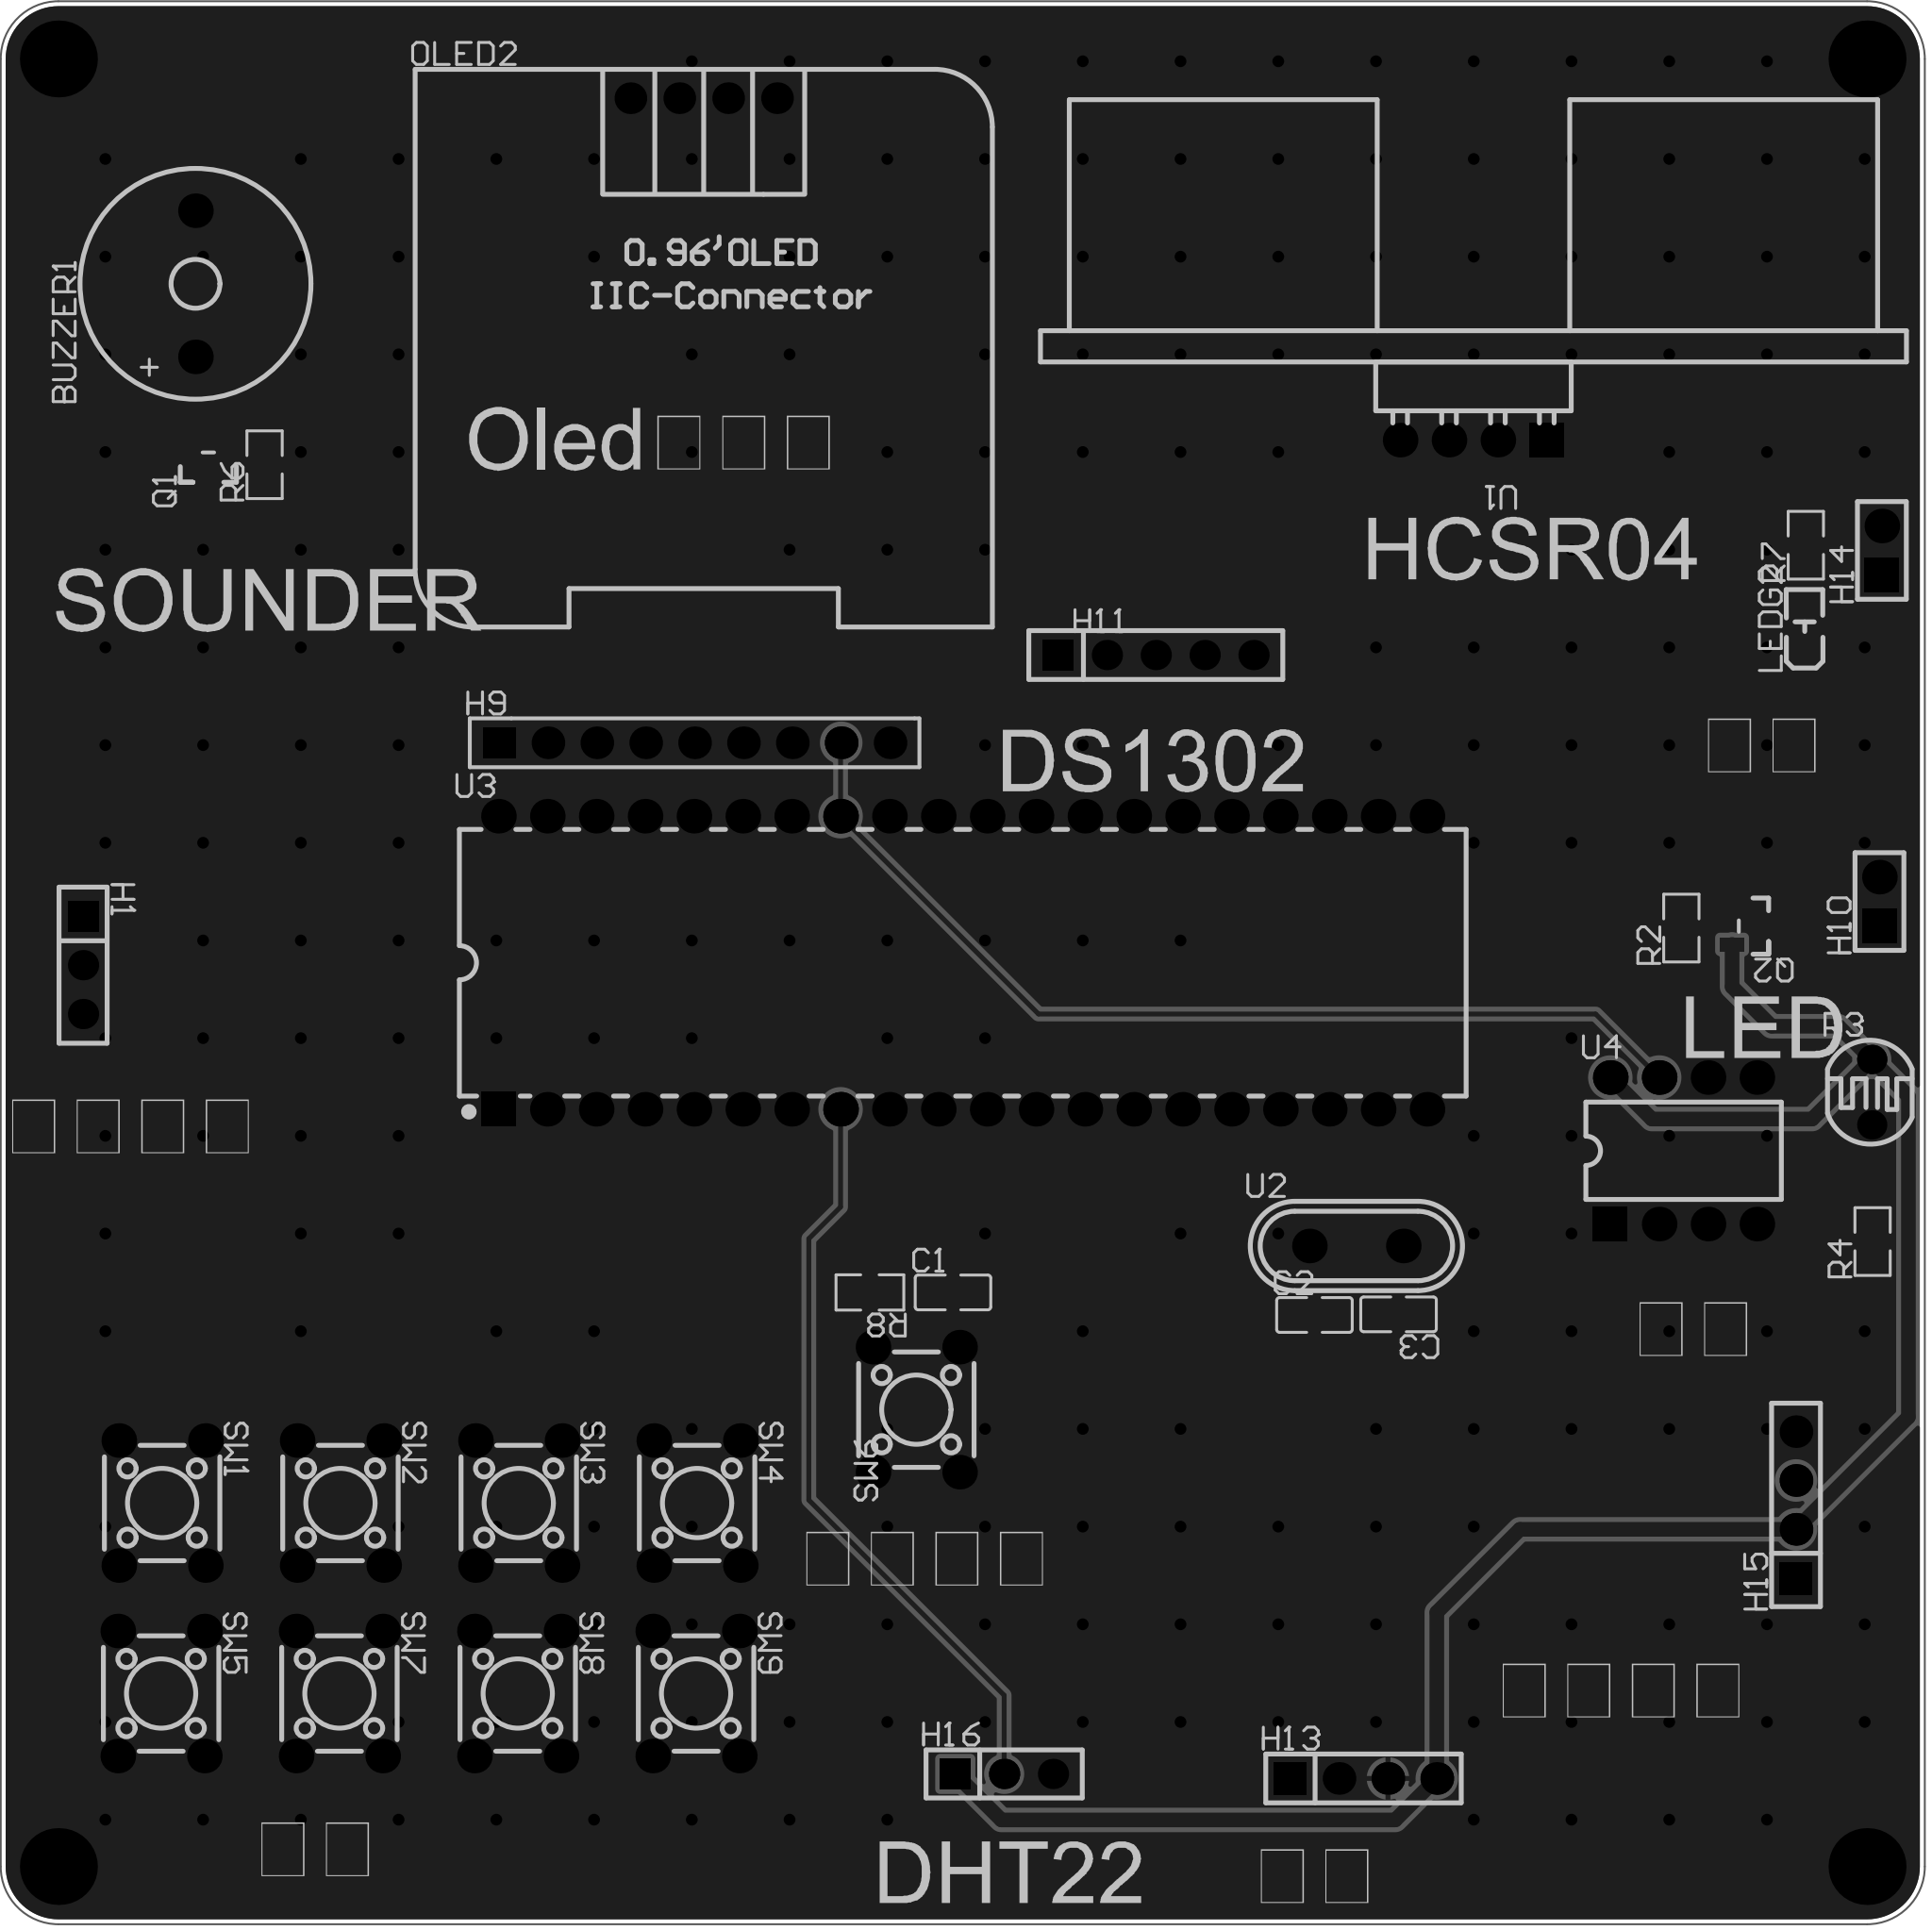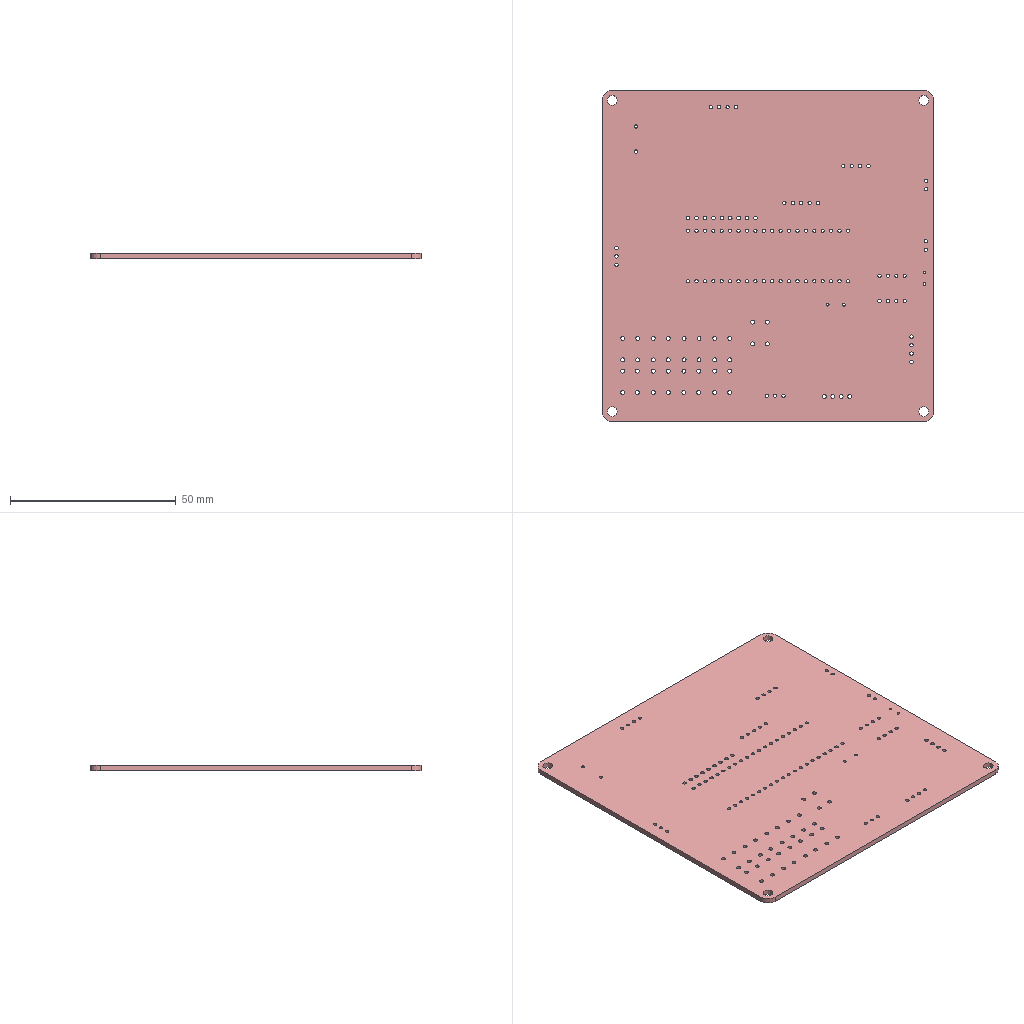Circuit board layout | Altium Designer | box 100 x 100 x 1.6 mm
Layer stack:
# Altium Designer layer stack of  (unit mm; dielectric type: 0 none, 1 core, 2 prepreg, 3 surface material)
index,name,kind,layer,copper_thickness_mm,dielectric_type,dielectric_thickness_mm,dielectric_material,dielectric_constant
0,Top Paste Mask Layer,other,,,,,,
1,Top Silkscreen Layer,other,,,,,,
2,Top Solder Mask Layer,dielectric,,,3,0.01,,3.3
3,Top Layer,copper,Top Layer,0.035,,,,
4,Dielectric1,dielectric,,,3,1.51,FR4,4.5
5,Bottom Layer,copper,Bottom Layer,0.035,,,,
6,Bottom Solder Mask Layer,dielectric,,,3,0.01,,3.3
7,Bottom Silkscreen Layer,other,,,,,,
8,Bottom Paste Mask Layer,other,,,,,,
# drill layer pairs: low layer,high layer
drill_pair,Top Layer,Bottom Layer
Part placement:
Designator,Comment,Layer,Footprint,Center-X(mm),Center-Y(mm),Rotation
SW1,,TopLayer,SW-TH_4P-L6.0-W6.0-P4.50-LS6.5,99.74,102.841,270
SW2,,TopLayer,SW-TH_4P-L6.0-W6.0-P4.50-LS6.5,109.007,102.841,270
SW3,,TopLayer,SW-TH_4P-L6.0-W6.0-P4.50-LS6.5,118.275,102.841,270
SW4,,TopLayer,SW-TH_4P-L6.0-W6.0-P4.50-LS6.5,127.543,102.841,270
OLED2,,TopLayer,0.96OLED_4P,127.889,175.895,0
BUZZER1,buzzer-12X9,TopLayer,BUZ-TH_BD12.0-P7.60-D0.6-FD,101.473,166.243,90
C1,10uf,TopLayer,C0805,140.843,113.792,0
C2,30pf,TopLayer,C0805,159.629,112.62,0
C3,30pf,TopLayer,C0805,164,112.652,180
H9,,TopLayer,HDR-TH_9P-P2.54-V-F-1,127.414,142.375,0
H13,,TopLayer,HDR-TH_4P-P2.54-V-M,162.179,88.519,0
H14,,TopLayer,HDR-TH_2P-P2.54-V-M-1,189.121,152.379,90
LEDG2,,TopLayer,LED_0805,185.106,148.363,90
Q1,2N3906S-RTK/PS,TopLayer,SOT-23-3_L2.9-W1.3-P1.90-LS2.4-TR,102.143,156.573,90
R6,2.2K,TopLayer,R0805,105.064,156.835,90
R7,220,TopLayer,R0805,185.168,152.649,90
R8,10K,TopLayer,R0805,136.525,113.792,180
U2,11.059MHz,TopLayer,HC-49US_L11.0-W4.6-P4.88,161.809,116.208,0
U3,STC89C516RD+40I-PDIP40,TopLayer,DIP-40_L52.3-W13.9-P2.54-LS15.2-BL,141.351,130.937,0
H1,,TopLayer,HDR-TH_3P-P2.54-V-F,95.631,130.81,270
H10,,TopLayer,HDR-TH_2P-P2.54-V-M-1,188.994,134.12,90
H15,,TopLayer,HDR-TH_4P-P2.54-V-F,184.658,102.743,90
H16,,TopLayer,HDR-TH_3P-P2.54-V-F,143.502,88.753,0
U1,HC-SR04,TopLayer,TH_HC-SR04V,167.894,158.115,180
Q2,,TopLayer,S8550P_SOT,182.584,132.842,180
H11,,TopLayer,HDR-TH_5P-P2.54-V-F,151.384,146.939,0
R2,1K,TopLayer,R0805,178.698,132.739,90
R3,GL5549(80-100),TopLayer,RES-TH_L5.1-W4.3-P3.40-D0.5,188.595,124.206,0
R4,10K,TopLayer,R0805,188.637,116.438,90
SW5,,TopLayer,SW-TH_4P-L6.0-W6.0-P4.50-LS6.5,99.687,92.935,270
SW6,,TopLayer,SW-TH_4P-L6.0-W6.0-P4.50-LS6.5,138.938,107.696,90
SW7,,TopLayer,SW-TH_4P-L6.0-W6.0-P4.50-LS6.5,108.954,92.935,270
SW8,,TopLayer,SW-TH_4P-L6.0-W6.0-P4.50-LS6.5,118.222,92.935,270
SW9,,TopLayer,SW-TH_4P-L6.0-W6.0-P4.50-LS6.5,127.49,92.935,270
U4,ADC0832CCN,TopLayer,DIP-8_L9.7-W6.4-P2.54-LS7.6-BL,178.816,121.158,0
Pad and via stacks:
# Altium Designer via and pad stacks of  (unit mm). Each distinct definition once, with the count of objects using it.
# via: kind,start_layer,end_layer,hole_mm,diameter_mm,mode(0 simple;1 top-mid-bottom;2 full stack),diameter_per_layer,count,example_net
# pad: kind,layer,hole_mm,hole_type(0 round;1 square;2 slot),plating,top_size,top_shape(1 round;2 rect;3 octagon;9 rounded rect),mid_size,bottom_size,mode,footprint,size_per_layer,count,example
pad,Multi-Layer,3,0,plated,4x4,1,4x4,4x4,0,,,4,1
pad,Multi-Layer,1.2,0,plated,1.8x1.8,1,1.8x1.8,1.8x1.8,0,SW-TH_4P-L6.0-W6.0-P4.50-LS6.5,,36,SW1.1
pad,Multi-Layer,1,0,plated,1.65x1.65,1,1.65x1.65,1.65x1.65,0,0.96OLED_4P,,4,OLED2.4
pad,Multi-Layer,1,0,plated,1.8x1.8,1,1.8x1.8,1.8x1.8,0,BUZ-TH_BD12.0-P7.60-D0.6-FD,,2,BUZZER1.2
pad,Multi-Layer,1.1,0,plated,1.7x1.575,2,1.7x1.575,1.7x1.575,0,HDR-TH_9P-P2.54-V-F-1,,1,H9.1
pad,Multi-Layer,1.1,0,plated,1.7x1.7,1,1.7x1.7,1.7x1.7,0,HDR-TH_9P-P2.54-V-F-1,,8,H9.2
pad,Multi-Layer,1.1,0,plated,1.7x1.7,2,1.7x1.7,1.7x1.7,0,HDR-TH_4P-P2.54-V-M,,1,H13.1
pad,Multi-Layer,1.1,0,plated,1.7x1.7,1,1.7x1.7,1.7x1.7,0,HDR-TH_4P-P2.54-V-M,,3,H13.2
pad,Multi-Layer,1,0,plated,1.8x1.8,1,1.8x1.8,1.8x1.8,0,HDR-TH_2P-P2.54-V-M-1,,2,H14.2
pad,Multi-Layer,1,0,plated,1.8x1.8,2,1.8x1.8,1.8x1.8,0,HDR-TH_2P-P2.54-V-M-1,,2,H14.1
pad,Multi-Layer,0.8,0,plated,1.8x1.8,1,1.8x1.8,1.8x1.8,0,HC-49US_L11.0-W4.6-P4.88,,2,U2.1
pad,Multi-Layer,1,0,plated,1.8x1.8,1,1.8x1.8,1.8x1.8,0,DIP-40_L52.3-W13.9-P2.54-LS15.2-BL,,39,U3.19
pad,Multi-Layer,1,0,plated,1.8x1.8,2,1.8x1.8,1.8x1.8,0,DIP-40_L52.3-W13.9-P2.54-LS15.2-BL,,1,U3.1
pad,Multi-Layer,1.02,0,plated,1.575x1.575,1,1.575x1.575,1.575x1.575,0,HDR-TH_3P-P2.54-V-F,,4,H1.3
pad,Multi-Layer,1.02,0,plated,1.575x1.575,2,1.575x1.575,1.575x1.575,0,HDR-TH_3P-P2.54-V-F,,2,H1.1
pad,Multi-Layer,1.1,0,plated,1.7x1.7,2,1.7x1.7,1.7x1.7,0,HDR-TH_4P-P2.54-V-F,,1,H15.1
pad,Multi-Layer,1.1,0,plated,1.7x1.7,1,1.7x1.7,1.7x1.7,0,HDR-TH_4P-P2.54-V-F,,3,H15.2
pad,Multi-Layer,1.001,0,plated,1.8x1.8,1,1.8x1.8,1.8x1.8,0,TH_HC-SR04V,,3,U1.4
pad,Multi-Layer,1.001,0,plated,1.8x1.8,2,1.8x1.8,1.8x1.8,0,TH_HC-SR04V,,1,U1.1
pad,Multi-Layer,1.02,0,plated,1.575x1.575,1,1.575x1.575,1.575x1.575,0,HDR-TH_5P-P2.54-V-F,,4,H11.5
pad,Multi-Layer,1.02,0,plated,1.575x1.575,2,1.575x1.575,1.575x1.575,0,HDR-TH_5P-P2.54-V-F,,1,H11.1
pad,Multi-Layer,0.762,0,plated,1.524x1.524,1,1.524x1.524,1.524x1.524,0,RES-TH_L5.1-W4.3-P3.40-D0.5,,2,R3.2
pad,Multi-Layer,1,0,plated,1.8x1.8,2,1.8x1.8,1.8x1.8,0,DIP-8_L9.7-W6.4-P2.54-LS7.6-BL,,1,U4.1
pad,Multi-Layer,1,0,plated,1.8x1.8,1,1.8x1.8,1.8x1.8,0,DIP-8_L9.7-W6.4-P2.54-LS7.6-BL,,7,U4.2
pad,Top Layer,0,0,plated,1.41x1.35,2,1.41x1.35,1.41x1.35,0,C0805,,6,C1.2
pad,Top Layer,0,0,plated,1x1.25,2,1x1.25,1x1.25,0,LED_0805,,2,LEDG2.2
pad,Top Layer,0,0,plated,0.7x1.25,2,0.7x1.25,0.7x1.25,0,SOT-23-3_L2.9-W1.3-P1.90-LS2.4-TR,,3,Q1.3
pad,Top Layer,0,0,plated,1.133x1.377,2,1.133x1.377,1.133x1.377,0,R0805,,10,R6.2
pad,Top Layer,0,0,plated,0.701x1.25,2,0.701x1.25,0.701x1.25,0,S8550P_SOT,,3,Q2.3
via,Top Layer,Bottom Layer,0.3048,0.61,0,,232,GND
Copper pours:
name,layer,net,type(0 solid;1 hatched;2 none)
Bottom Layer-GND,Bottom Layer,GND,0
Top Layer-GND,Top Layer,GND,0
Design rules, without the lines most boards share:
# Altium Designer design rules of  (exported by Altium Designer, unit mm)
# columns: name | kind | enabled | priority | scope1 | scope2 | descriptor | typed fields (field=value)
Copper_copperRegion_copperThickness1oz | 0 | disabled | 4 | All | All | Clearance Constraint (Gap=5.984mil) (Disabled)(All),(All) | gap=0.152
Copper_copperRegion_copperThickness1oz_1 | 63 | disabled | 4 | All | All | Board Clearance Constraint (Gap=0mil) (Disabled)(All) |
Copper_copperRegion_Copper_copperRegion | 0 | disabled | 5 | All | All | Clearance Constraint (Gap=5.984mil) (Disabled)(All),(All) | gap=0.152
Copper_copperRegion_Copper_copperRegion_1 | 63 | disabled | 5 | All | All | Board Clearance Constraint (Gap=0mil) (Disabled)(All) |
copperThickness1oz | 0 | enabled | 6 | All | All | Clearance Constraint (Gap=5.984mil) (All),(All) | gap=0.152
copperThickness1oz_1 | 63 | enabled | 6 | All | All | Board Clearance Constraint (Gap=0mil) (All) |
copperRegion_copperThickness1oz | 20 | disabled | 1 | All | All | Polygon Connect Rule(Relief Connect )(Conductor Width=10mil) (Relief Angle=90 Angle) (Entries=4) (Air Gap Width=10mil) (Disabled)(All),(All) | connect_style(0=relief,1=direct,2=none)=0 relief_conductor_width=0.254 relief_entries=4
copperRegion_Copper_copperRegion | 20 | disabled | 2 | All | All | Polygon Connect Rule(Relief Connect )(Conductor Width=10mil) (Relief Angle=90 Angle) (Entries=4) (Air Gap Width=10mil) (Disabled)(All),(All) | connect_style(0=relief,1=direct,2=none)=0 relief_conductor_width=0.254 relief_entries=4
copperRegion | 20 | enabled | 3 | All | All | Polygon Connect Rule(Relief Connect )(Conductor Width=10mil) (Relief Angle=90 Angle) (Entries=4) (Air Gap Width=10mil) (All),(All) | connect_style(0=relief,1=direct,2=none)=0 relief_conductor_width=0.254 relief_entries=4